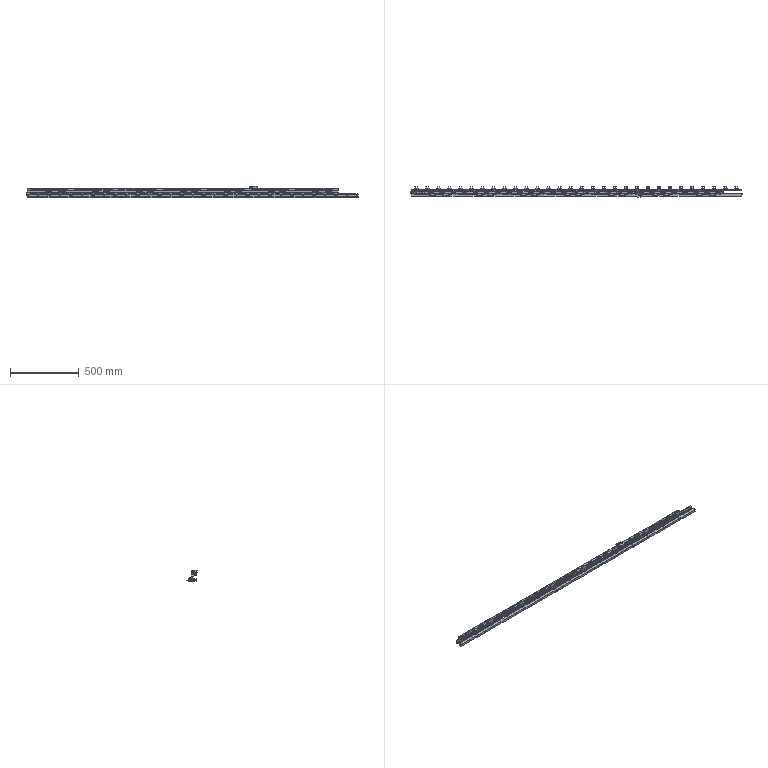Part | NX | 602 solids | 22113 faces | volume 3015794 mm3 | plane 12046 | cylinder 7143 | cone 2610 | torus 224 | sphere 90 | commonest cylinder face diameters 3 x1310 4 x936 2.5 x818 3.3 x590 3.5 x504 6 x308